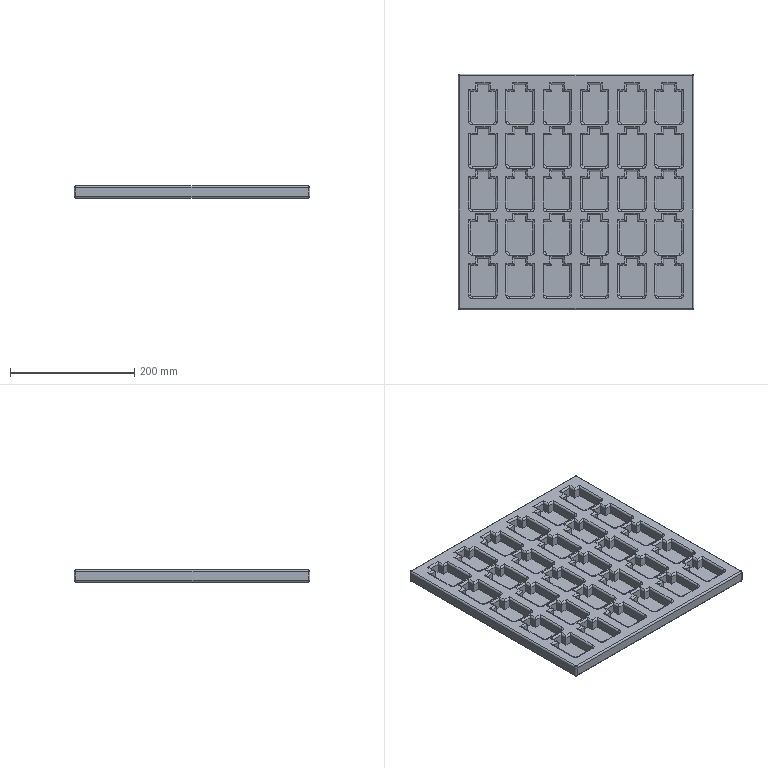Part | SolidWorks | features Fillet 3, ICE 2, Extrusion 1, LPattern 1 | 1 solid | 656 faces | box 380 x 380 x 20 mm | volume 1730652 mm3 | cylinder 312 | plane 276 | torus 60 | sphere 8 | commonest cylinder face diameters 6 x312